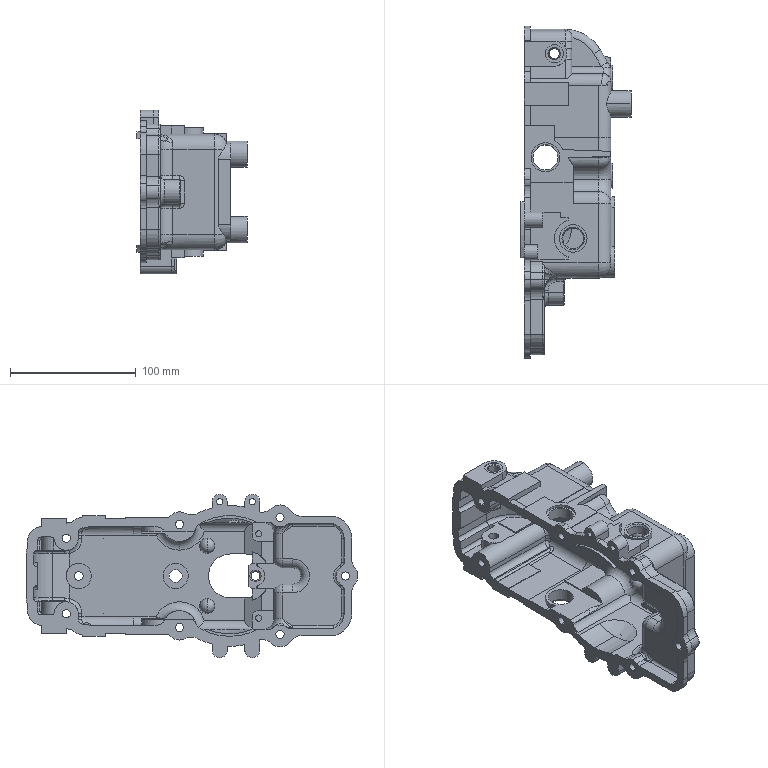Part | SolidWorks | features BaseBody 1 | 1 solid | 702 faces | box 87.5 x 264 x 130 mm | volume 333498 mm3 | cylinder 301 | plane 252 | torus 61 | cone 44 | spline 28 | sphere 16 | commonest cylinder face diameters 20 x57 12 x25 6 x24 5 x16 6.5 x14 10 x14